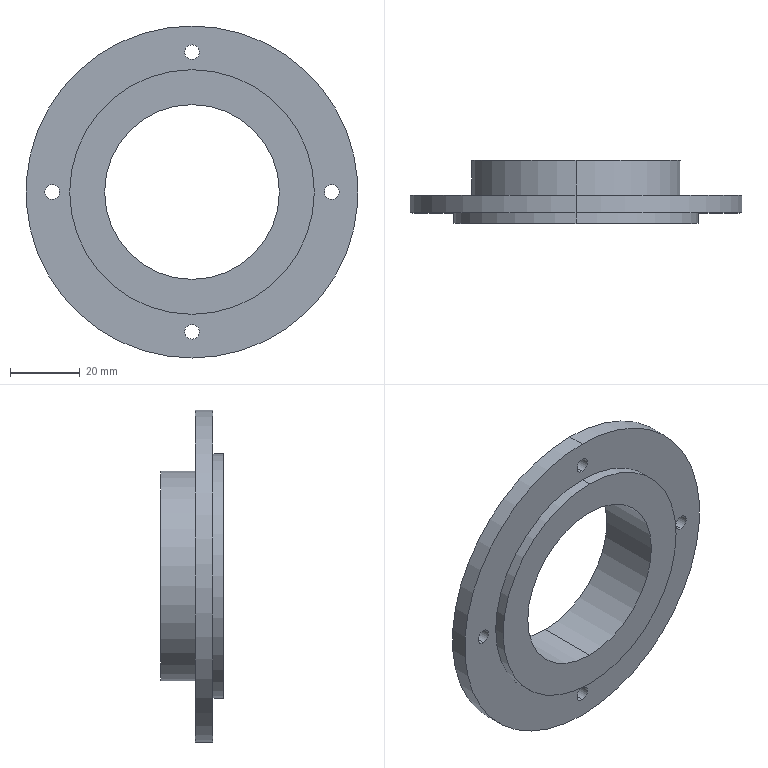Part | STEP file | Rotating Shaft | 1 solid | 20 faces | box 95 x 18 x 95 mm | volume 39641 mm3 | cylinder 16 | plane 4 | commonest cylinder face diameters 4.2 x8 50 x2 60 x2 70 x2 95 x2
STEP:
#1=CARTESIAN_POINT('',(0.,8.,47.5));
#2=VERTEX_POINT('',#1);
#3=CARTESIAN_POINT('',(0.,8.,-47.5));
#4=VERTEX_POINT('',#3);
#5=CARTESIAN_POINT('',(0.,8.,0.));
#6=DIRECTION('',(0.,1.,0.));
#7=DIRECTION('',(0.,0.,-1.));
#8=AXIS2_PLACEMENT_3D('',#5,#6,#7);
#9=CIRCLE('',#8,47.5);
#10=EDGE_CURVE('',#2,#4,#9,.T.);
#11=ORIENTED_EDGE('',*,*,#10,.F.);
#12=CARTESIAN_POINT('',(0.,3.,47.5));
#13=VERTEX_POINT('',#12);
#14=CARTESIAN_POINT('',(0.,0.,47.5));
#15=DIRECTION('',(0.,-1.,0.));
#16=VECTOR('',#15,1000.);
#17=LINE('',#14,#16);
#18=EDGE_CURVE('',#2,#13,#17,.T.);
#19=ORIENTED_EDGE('',*,*,#18,.T.);
#20=CARTESIAN_POINT('',(0.,3.,-47.5));
#21=VERTEX_POINT('',#20);
#22=CARTESIAN_POINT('',(0.,3.,0.));
#23=DIRECTION('',(0.,1.,0.));
#24=DIRECTION('',(0.,0.,-1.));
#25=AXIS2_PLACEMENT_3D('',#22,#23,#24);
#26=CIRCLE('',#25,47.5);
#27=EDGE_CURVE('',#13,#21,#26,.T.);
#28=ORIENTED_EDGE('',*,*,#27,.T.);
#29=CARTESIAN_POINT('',(0.,0.,-47.5));
#30=DIRECTION('',(0.,-1.,0.));
#31=VECTOR('',#30,1000.);
#32=LINE('',#29,#31);
#33=EDGE_CURVE('',#4,#21,#32,.T.);
#34=ORIENTED_EDGE('',*,*,#33,.F.);
#35=EDGE_LOOP('',(#11,#19,#28,#34));
#36=FACE_OUTER_BOUND('',#35,.T.);
#37=CARTESIAN_POINT('',(0.,0.,0.));
#38=DIRECTION('',(0.,-1.,0.));
#39=DIRECTION('',(0.,0.,-1.));
#40=AXIS2_PLACEMENT_3D('',#37,#38,#39);
#41=CYLINDRICAL_SURFACE('',#40,47.5);
#42=ADVANCED_FACE('',(#36),#41,.T.);
#43=CARTESIAN_POINT('',(0.,18.,-30.));
#44=VERTEX_POINT('',#43);
#45=CARTESIAN_POINT('',(0.,18.,30.));
#46=VERTEX_POINT('',#45);
#47=CARTESIAN_POINT('',(0.,18.,0.));
#48=DIRECTION('',(0.,-1.,0.));
#49=DIRECTION('',(0.,0.,-1.));
#50=AXIS2_PLACEMENT_3D('',#47,#48,#49);
#51=CIRCLE('',#50,30.);
#52=EDGE_CURVE('',#44,#46,#51,.T.);
#53=ORIENTED_EDGE('',*,*,#52,.T.);
#54=CARTESIAN_POINT('',(0.,8.,30.));
#55=VERTEX_POINT('',#54);
#56=CARTESIAN_POINT('',(0.,0.,30.));
#57=DIRECTION('',(0.,-1.,0.));
#58=VECTOR('',#57,1000.);
#59=LINE('',#56,#58);
#60=EDGE_CURVE('',#46,#55,#59,.T.);
#61=ORIENTED_EDGE('',*,*,#60,.T.);
#62=CARTESIAN_POINT('',(0.,8.,-30.));
#63=VERTEX_POINT('',#62);
#64=CARTESIAN_POINT('',(0.,8.,0.));
#65=DIRECTION('',(0.,-1.,0.));
#66=DIRECTION('',(0.,0.,-1.));
#67=AXIS2_PLACEMENT_3D('',#64,#65,#66);
#68=CIRCLE('',#67,30.);
#69=EDGE_CURVE('',#63,#55,#68,.T.);
#70=ORIENTED_EDGE('',*,*,#69,.F.);
#71=CARTESIAN_POINT('',(0.,0.,-30.));
#72=DIRECTION('',(0.,-1.,0.));
#73=VECTOR('',#72,1000.);
#74=LINE('',#71,#73);
#75=EDGE_CURVE('',#44,#63,#74,.T.);
#76=ORIENTED_EDGE('',*,*,#75,.F.);
#77=EDGE_LOOP('',(#53,#61,#70,#76));
#78=FACE_OUTER_BOUND('',#77,.T.);
#79=CARTESIAN_POINT('',(0.,0.,0.));
#80=DIRECTION('',(0.,-1.,0.));
#81=DIRECTION('',(0.,0.,-1.));
#82=AXIS2_PLACEMENT_3D('',#79,#80,#81);
#83=CYLINDRICAL_SURFACE('',#82,30.);
#84=ADVANCED_FACE('',(#78),#83,.T.);
#85=CARTESIAN_POINT('',(0.,3.,37.9));
#86=VERTEX_POINT('',#85);
#87=CARTESIAN_POINT('',(0.,3.,42.1));
#88=VERTEX_POINT('',#87);
#89=CARTESIAN_POINT('',(0.,3.,40.));
#90=DIRECTION('',(0.,1.,0.));
#91=DIRECTION('',(0.,0.,1.));
#92=AXIS2_PLACEMENT_3D('',#89,#90,#91);
#93=CIRCLE('',#92,2.1);
#94=EDGE_CURVE('',#86,#88,#93,.T.);
#95=ORIENTED_EDGE('',*,*,#94,.F.);
#96=CARTESIAN_POINT('',(0.,8.,37.9));
#97=VERTEX_POINT('',#96);
#98=CARTESIAN_POINT('',(0.,3.,37.9));
#99=DIRECTION('',(0.,1.,0.));
#100=VECTOR('',#99,1000.);
#101=LINE('',#98,#100);
#102=EDGE_CURVE('',#86,#97,#101,.T.);
#103=ORIENTED_EDGE('',*,*,#102,.T.);
#104=CARTESIAN_POINT('',(0.,8.,42.1));
#105=VERTEX_POINT('',#104);
#106=CARTESIAN_POINT('',(0.,8.,40.));
#107=DIRECTION('',(0.,-1.,0.));
#108=DIRECTION('',(0.,0.,1.));
#109=AXIS2_PLACEMENT_3D('',#106,#107,#108);
#110=CIRCLE('',#109,2.1);
#111=EDGE_CURVE('',#105,#97,#110,.T.);
#112=ORIENTED_EDGE('',*,*,#111,.F.);
#113=CARTESIAN_POINT('',(0.,3.,42.1));
#114=DIRECTION('',(0.,1.,0.));
#115=VECTOR('',#114,1000.);
#116=LINE('',#113,#115);
#117=EDGE_CURVE('',#88,#105,#116,.T.);
#118=ORIENTED_EDGE('',*,*,#117,.F.);
#119=EDGE_LOOP('',(#95,#103,#112,#118));
#120=FACE_OUTER_BOUND('',#119,.T.);
#121=CARTESIAN_POINT('',(0.,3.,40.));
#122=DIRECTION('',(0.,1.,0.));
#123=DIRECTION('',(0.,0.,1.));
#124=AXIS2_PLACEMENT_3D('',#121,#122,#123);
#125=CYLINDRICAL_SURFACE('',#124,2.1);
#126=ADVANCED_FACE('',(#120),#125,.F.);
#127=CARTESIAN_POINT('',(-40.,3.,-2.1));
#128=VERTEX_POINT('',#127);
#129=CARTESIAN_POINT('',(-40.,3.,2.1));
#130=VERTEX_POINT('',#129);
#131=CARTESIAN_POINT('',(-40.,3.,0.));
#132=DIRECTION('',(0.,1.,0.));
#133=DIRECTION('',(0.,0.,1.));
#134=AXIS2_PLACEMENT_3D('',#131,#132,#133);
#135=CIRCLE('',#134,2.1);
#136=EDGE_CURVE('',#128,#130,#135,.T.);
#137=ORIENTED_EDGE('',*,*,#136,.F.);
#138=CARTESIAN_POINT('',(-40.,8.,-2.1));
#139=VERTEX_POINT('',#138);
#140=CARTESIAN_POINT('',(-40.,3.,-2.1));
#141=DIRECTION('',(0.,1.,0.));
#142=VECTOR('',#141,1000.);
#143=LINE('',#140,#142);
#144=EDGE_CURVE('',#128,#139,#143,.T.);
#145=ORIENTED_EDGE('',*,*,#144,.T.);
#146=CARTESIAN_POINT('',(-40.,8.,2.1));
#147=VERTEX_POINT('',#146);
#148=CARTESIAN_POINT('',(-40.,8.,0.));
#149=DIRECTION('',(0.,-1.,0.));
#150=DIRECTION('',(0.,0.,1.));
#151=AXIS2_PLACEMENT_3D('',#148,#149,#150);
#152=CIRCLE('',#151,2.1);
#153=EDGE_CURVE('',#147,#139,#152,.T.);
#154=ORIENTED_EDGE('',*,*,#153,.F.);
#155=CARTESIAN_POINT('',(-40.,3.,2.1));
#156=DIRECTION('',(0.,1.,0.));
#157=VECTOR('',#156,1000.);
#158=LINE('',#155,#157);
#159=EDGE_CURVE('',#130,#147,#158,.T.);
#160=ORIENTED_EDGE('',*,*,#159,.F.);
#161=EDGE_LOOP('',(#137,#145,#154,#160));
#162=FACE_OUTER_BOUND('',#161,.T.);
#163=CARTESIAN_POINT('',(-40.,3.,0.));
#164=DIRECTION('',(0.,1.,0.));
#165=DIRECTION('',(0.,0.,1.));
#166=AXIS2_PLACEMENT_3D('',#163,#164,#165);
#167=CYLINDRICAL_SURFACE('',#166,2.1);
#168=ADVANCED_FACE('',(#162),#167,.F.);
#169=CARTESIAN_POINT('',(0.,3.,-42.1));
#170=VERTEX_POINT('',#169);
#171=CARTESIAN_POINT('',(0.,3.,-37.9));
#172=VERTEX_POINT('',#171);
#173=CARTESIAN_POINT('',(0.,3.,-40.));
#174=DIRECTION('',(0.,1.,0.));
#175=DIRECTION('',(0.,0.,1.));
#176=AXIS2_PLACEMENT_3D('',#173,#174,#175);
#177=CIRCLE('',#176,2.1);
#178=EDGE_CURVE('',#170,#172,#177,.T.);
#179=ORIENTED_EDGE('',*,*,#178,.F.);
#180=CARTESIAN_POINT('',(0.,8.,-42.1));
#181=VERTEX_POINT('',#180);
#182=CARTESIAN_POINT('',(0.,3.,-42.1));
#183=DIRECTION('',(0.,1.,0.));
#184=VECTOR('',#183,1000.);
#185=LINE('',#182,#184);
#186=EDGE_CURVE('',#170,#181,#185,.T.);
#187=ORIENTED_EDGE('',*,*,#186,.T.);
#188=CARTESIAN_POINT('',(0.,8.,-37.9));
#189=VERTEX_POINT('',#188);
#190=CARTESIAN_POINT('',(0.,8.,-40.));
#191=DIRECTION('',(0.,-1.,0.));
#192=DIRECTION('',(0.,0.,1.));
#193=AXIS2_PLACEMENT_3D('',#190,#191,#192);
#194=CIRCLE('',#193,2.1);
#195=EDGE_CURVE('',#189,#181,#194,.T.);
#196=ORIENTED_EDGE('',*,*,#195,.F.);
#197=CARTESIAN_POINT('',(0.,3.,-37.9));
#198=DIRECTION('',(0.,1.,0.));
#199=VECTOR('',#198,1000.);
#200=LINE('',#197,#199);
#201=EDGE_CURVE('',#172,#189,#200,.T.);
#202=ORIENTED_EDGE('',*,*,#201,.F.);
#203=EDGE_LOOP('',(#179,#187,#196,#202));
#204=FACE_OUTER_BOUND('',#203,.T.);
#205=CARTESIAN_POINT('',(0.,3.,-40.));
#206=DIRECTION('',(0.,1.,0.));
#207=DIRECTION('',(0.,0.,1.));
#208=AXIS2_PLACEMENT_3D('',#205,#206,#207);
#209=CYLINDRICAL_SURFACE('',#208,2.1);
#210=ADVANCED_FACE('',(#204),#209,.F.);
#211=CARTESIAN_POINT('',(40.,3.,-2.1));
#212=VERTEX_POINT('',#211);
#213=CARTESIAN_POINT('',(40.,3.,2.1));
#214=VERTEX_POINT('',#213);
#215=CARTESIAN_POINT('',(40.,3.,0.));
#216=DIRECTION('',(0.,1.,0.));
#217=DIRECTION('',(0.,0.,1.));
#218=AXIS2_PLACEMENT_3D('',#215,#216,#217);
#219=CIRCLE('',#218,2.1);
#220=EDGE_CURVE('',#212,#214,#219,.T.);
#221=ORIENTED_EDGE('',*,*,#220,.F.);
#222=CARTESIAN_POINT('',(40.,8.,-2.1));
#223=VERTEX_POINT('',#222);
#224=CARTESIAN_POINT('',(40.,3.,-2.1));
#225=DIRECTION('',(0.,1.,0.));
#226=VECTOR('',#225,1000.);
#227=LINE('',#224,#226);
#228=EDGE_CURVE('',#212,#223,#227,.T.);
#229=ORIENTED_EDGE('',*,*,#228,.T.);
#230=CARTESIAN_POINT('',(40.,8.,2.1));
#231=VERTEX_POINT('',#230);
#232=CARTESIAN_POINT('',(40.,8.,0.));
#233=DIRECTION('',(0.,-1.,0.));
#234=DIRECTION('',(0.,0.,1.));
#235=AXIS2_PLACEMENT_3D('',#232,#233,#234);
#236=CIRCLE('',#235,2.1);
#237=EDGE_CURVE('',#231,#223,#236,.T.);
#238=ORIENTED_EDGE('',*,*,#237,.F.);
#239=CARTESIAN_POINT('',(40.,3.,2.1));
#240=DIRECTION('',(0.,1.,0.));
#241=VECTOR('',#240,1000.);
#242=LINE('',#239,#241);
#243=EDGE_CURVE('',#214,#231,#242,.T.);
#244=ORIENTED_EDGE('',*,*,#243,.F.);
#245=EDGE_LOOP('',(#221,#229,#238,#244));
#246=FACE_OUTER_BOUND('',#245,.T.);
#247=CARTESIAN_POINT('',(40.,3.,0.));
#248=DIRECTION('',(0.,1.,0.));
#249=DIRECTION('',(0.,0.,1.));
#250=AXIS2_PLACEMENT_3D('',#247,#248,#249);
#251=CYLINDRICAL_SURFACE('',#250,2.1);
#252=ADVANCED_FACE('',(#246),#251,.F.);
#253=CARTESIAN_POINT('',(0.,3.,35.));
#254=VERTEX_POINT('',#253);
#255=CARTESIAN_POINT('',(0.,3.,-35.));
#256=VERTEX_POINT('',#255);
#257=CARTESIAN_POINT('',(0.,3.,0.));
#258=DIRECTION('',(0.,1.,0.));
#259=DIRECTION('',(0.,0.,-1.));
#260=AXIS2_PLACEMENT_3D('',#257,#258,#259);
#261=CIRCLE('',#260,35.);
#262=EDGE_CURVE('',#254,#256,#261,.T.);
#263=ORIENTED_EDGE('',*,*,#262,.F.);
#264=CARTESIAN_POINT('',(0.,0.,35.));
#265=VERTEX_POINT('',#264);
#266=CARTESIAN_POINT('',(0.,0.,35.));
#267=DIRECTION('',(0.,-1.,0.));
#268=VECTOR('',#267,1000.);
#269=LINE('',#266,#268);
#270=EDGE_CURVE('',#254,#265,#269,.T.);
#271=ORIENTED_EDGE('',*,*,#270,.T.);
#272=CARTESIAN_POINT('',(0.,0.,-35.));
#273=VERTEX_POINT('',#272);
#274=CARTESIAN_POINT('',(0.,0.,0.));
#275=DIRECTION('',(0.,1.,0.));
#276=DIRECTION('',(0.,0.,-1.));
#277=AXIS2_PLACEMENT_3D('',#274,#275,#276);
#278=CIRCLE('',#277,35.);
#279=EDGE_CURVE('',#265,#273,#278,.T.);
#280=ORIENTED_EDGE('',*,*,#279,.T.);
#281=CARTESIAN_POINT('',(0.,0.,-35.));
#282=DIRECTION('',(0.,-1.,0.));
#283=VECTOR('',#282,1000.);
#284=LINE('',#281,#283);
#285=EDGE_CURVE('',#256,#273,#284,.T.);
#286=ORIENTED_EDGE('',*,*,#285,.F.);
#287=EDGE_LOOP('',(#263,#271,#280,#286));
#288=FACE_OUTER_BOUND('',#287,.T.);
#289=CARTESIAN_POINT('',(0.,0.,0.));
#290=DIRECTION('',(0.,-1.,0.));
#291=DIRECTION('',(0.,0.,-1.));
#292=AXIS2_PLACEMENT_3D('',#289,#290,#291);
#293=CYLINDRICAL_SURFACE('',#292,35.);
#294=ADVANCED_FACE('',(#288),#293,.T.);
#295=CARTESIAN_POINT('',(0.,18.,25.));
#296=VERTEX_POINT('',#295);
#297=CARTESIAN_POINT('',(0.,18.,-25.));
#298=VERTEX_POINT('',#297);
#299=CARTESIAN_POINT('',(0.,18.,0.));
#300=DIRECTION('',(0.,-1.,0.));
#301=DIRECTION('',(0.,0.,-1.));
#302=AXIS2_PLACEMENT_3D('',#299,#300,#301);
#303=CIRCLE('',#302,25.);
#304=EDGE_CURVE('',#296,#298,#303,.T.);
#305=ORIENTED_EDGE('',*,*,#304,.F.);
#306=CARTESIAN_POINT('',(0.,0.,25.));
#307=VERTEX_POINT('',#306);
#308=CARTESIAN_POINT('',(0.,0.,25.));
#309=DIRECTION('',(0.,-1.,0.));
#310=VECTOR('',#309,1000.);
#311=LINE('',#308,#310);
#312=EDGE_CURVE('',#296,#307,#311,.T.);
#313=ORIENTED_EDGE('',*,*,#312,.T.);
#314=CARTESIAN_POINT('',(0.,0.,-25.));
#315=VERTEX_POINT('',#314);
#316=CARTESIAN_POINT('',(0.,0.,0.));
#317=DIRECTION('',(0.,1.,0.));
#318=DIRECTION('',(0.,0.,-1.));
#319=AXIS2_PLACEMENT_3D('',#316,#317,#318);
#320=CIRCLE('',#319,25.);
#321=EDGE_CURVE('',#315,#307,#320,.T.);
#322=ORIENTED_EDGE('',*,*,#321,.F.);
#323=CARTESIAN_POINT('',(0.,0.,-25.));
#324=DIRECTION('',(0.,-1.,0.));
#325=VECTOR('',#324,1000.);
#326=LINE('',#323,#325);
#327=EDGE_CURVE('',#298,#315,#326,.T.);
#328=ORIENTED_EDGE('',*,*,#327,.F.);
#329=EDGE_LOOP('',(#305,#313,#322,#328));
#330=FACE_OUTER_BOUND('',#329,.T.);
#331=CARTESIAN_POINT('',(0.,0.,0.));
#332=DIRECTION('',(0.,-1.,0.));
#333=DIRECTION('',(0.,0.,-1.));
#334=AXIS2_PLACEMENT_3D('',#331,#332,#333);
#335=CYLINDRICAL_SURFACE('',#334,25.);
#336=ADVANCED_FACE('',(#330),#335,.F.);
#337=CARTESIAN_POINT('',(0.,8.,0.));
#338=DIRECTION('',(0.,1.,0.));
#339=DIRECTION('',(0.,0.,-1.));
#340=AXIS2_PLACEMENT_3D('',#337,#338,#339);
#341=CIRCLE('',#340,47.5);
#342=EDGE_CURVE('',#4,#2,#341,.T.);
#343=ORIENTED_EDGE('',*,*,#342,.T.);
#344=ORIENTED_EDGE('',*,*,#10,.T.);
#345=EDGE_LOOP('',(#343,#344));
#346=FACE_OUTER_BOUND('',#345,.T.);
#347=ORIENTED_EDGE('',*,*,#69,.T.);
#348=CARTESIAN_POINT('',(0.,8.,0.));
#349=DIRECTION('',(0.,-1.,0.));
#350=DIRECTION('',(0.,0.,-1.));
#351=AXIS2_PLACEMENT_3D('',#348,#349,#350);
#352=CIRCLE('',#351,30.);
#353=EDGE_CURVE('',#55,#63,#352,.T.);
#354=ORIENTED_EDGE('',*,*,#353,.T.);
#355=EDGE_LOOP('',(#347,#354));
#356=FACE_BOUND('',#355,.T.);
#357=ORIENTED_EDGE('',*,*,#111,.T.);
#358=CARTESIAN_POINT('',(0.,8.,40.));
#359=DIRECTION('',(0.,-1.,0.));
#360=DIRECTION('',(0.,0.,1.));
#361=AXIS2_PLACEMENT_3D('',#358,#359,#360);
#362=CIRCLE('',#361,2.1);
#363=EDGE_CURVE('',#97,#105,#362,.T.);
#364=ORIENTED_EDGE('',*,*,#363,.T.);
#365=EDGE_LOOP('',(#357,#364));
#366=FACE_BOUND('',#365,.T.);
#367=ORIENTED_EDGE('',*,*,#153,.T.);
#368=CARTESIAN_POINT('',(-40.,8.,0.));
#369=DIRECTION('',(0.,-1.,0.));
#370=DIRECTION('',(0.,0.,1.));
#371=AXIS2_PLACEMENT_3D('',#368,#369,#370);
#372=CIRCLE('',#371,2.1);
#373=EDGE_CURVE('',#139,#147,#372,.T.);
#374=ORIENTED_EDGE('',*,*,#373,.T.);
#375=EDGE_LOOP('',(#367,#374));
#376=FACE_BOUND('',#375,.T.);
#377=ORIENTED_EDGE('',*,*,#195,.T.);
#378=CARTESIAN_POINT('',(0.,8.,-40.));
#379=DIRECTION('',(0.,-1.,0.));
#380=DIRECTION('',(0.,0.,1.));
#381=AXIS2_PLACEMENT_3D('',#378,#379,#380);
#382=CIRCLE('',#381,2.1);
#383=EDGE_CURVE('',#181,#189,#382,.T.);
#384=ORIENTED_EDGE('',*,*,#383,.T.);
#385=EDGE_LOOP('',(#377,#384));
#386=FACE_BOUND('',#385,.T.);
#387=ORIENTED_EDGE('',*,*,#237,.T.);
#388=CARTESIAN_POINT('',(40.,8.,0.));
#389=DIRECTION('',(0.,-1.,0.));
#390=DIRECTION('',(0.,0.,1.));
#391=AXIS2_PLACEMENT_3D('',#388,#389,#390);
#392=CIRCLE('',#391,2.1);
#393=EDGE_CURVE('',#223,#231,#392,.T.);
#394=ORIENTED_EDGE('',*,*,#393,.T.);
#395=EDGE_LOOP('',(#387,#394));
#396=FACE_BOUND('',#395,.T.);
#397=CARTESIAN_POINT('',(47.5,8.,0.));
#398=DIRECTION('',(0.,1.,0.));
#399=DIRECTION('',(0.,0.,1.));
#400=AXIS2_PLACEMENT_3D('',#397,#398,#399);
#401=PLANE('',#400);
#402=ADVANCED_FACE('',(#346,#356,#366,#376,#386,#396),#401,.T.);
#403=ORIENTED_EDGE('',*,*,#18,.F.);
#404=ORIENTED_EDGE('',*,*,#342,.F.);
#405=ORIENTED_EDGE('',*,*,#33,.T.);
#406=CARTESIAN_POINT('',(0.,3.,0.));
#407=DIRECTION('',(0.,1.,0.));
#408=DIRECTION('',(0.,0.,-1.));
#409=AXIS2_PLACEMENT_3D('',#406,#407,#408);
#410=CIRCLE('',#409,47.5);
#411=EDGE_CURVE('',#21,#13,#410,.T.);
#412=ORIENTED_EDGE('',*,*,#411,.T.);
#413=EDGE_LOOP('',(#403,#404,#405,#412));
#414=FACE_OUTER_BOUND('',#413,.T.);
#415=CARTESIAN_POINT('',(0.,0.,0.));
#416=DIRECTION('',(0.,-1.,0.));
#417=DIRECTION('',(0.,0.,-1.));
#418=AXIS2_PLACEMENT_3D('',#415,#416,#417);
#419=CYLINDRICAL_SURFACE('',#418,47.5);
#420=ADVANCED_FACE('',(#414),#419,.T.);
#421=ORIENTED_EDGE('',*,*,#60,.F.);
#422=CARTESIAN_POINT('',(0.,18.,0.));
#423=DIRECTION('',(0.,-1.,0.));
#424=DIRECTION('',(0.,0.,-1.));
#425=AXIS2_PLACEMENT_3D('',#422,#423,#424);
#426=CIRCLE('',#425,30.);
#427=EDGE_CURVE('',#46,#44,#426,.T.);
#428=ORIENTED_EDGE('',*,*,#427,.T.);
#429=ORIENTED_EDGE('',*,*,#75,.T.);
#430=ORIENTED_EDGE('',*,*,#353,.F.);
#431=EDGE_LOOP('',(#421,#428,#429,#430));
#432=FACE_OUTER_BOUND('',#431,.T.);
#433=CARTESIAN_POINT('',(0.,0.,0.));
#434=DIRECTION('',(0.,-1.,0.));
#435=DIRECTION('',(0.,0.,-1.));
#436=AXIS2_PLACEMENT_3D('',#433,#434,#435);
#437=CYLINDRICAL_SURFACE('',#436,30.);
#438=ADVANCED_FACE('',(#432),#437,.T.);
#439=ORIENTED_EDGE('',*,*,#102,.F.);
#440=CARTESIAN_POINT('',(0.,3.,40.));
#441=DIRECTION('',(0.,1.,0.));
#442=DIRECTION('',(0.,0.,1.));
#443=AXIS2_PLACEMENT_3D('',#440,#441,#442);
#444=CIRCLE('',#443,2.1);
#445=EDGE_CURVE('',#88,#86,#444,.T.);
#446=ORIENTED_EDGE('',*,*,#445,.F.);
#447=ORIENTED_EDGE('',*,*,#117,.T.);
#448=ORIENTED_EDGE('',*,*,#363,.F.);
#449=EDGE_LOOP('',(#439,#446,#447,#448));
#450=FACE_OUTER_BOUND('',#449,.T.);
#451=CARTESIAN_POINT('',(0.,3.,40.));
#452=DIRECTION('',(0.,1.,0.));
#453=DIRECTION('',(0.,0.,1.));
#454=AXIS2_PLACEMENT_3D('',#451,#452,#453);
#455=CYLINDRICAL_SURFACE('',#454,2.1);
#456=ADVANCED_FACE('',(#450),#455,.F.);
#457=ORIENTED_EDGE('',*,*,#144,.F.);
#458=CARTESIAN_POINT('',(-40.,3.,0.));
#459=DIRECTION('',(0.,1.,0.));
#460=DIRECTION('',(0.,0.,1.));
#461=AXIS2_PLACEMENT_3D('',#458,#459,#460);
#462=CIRCLE('',#461,2.1);
#463=EDGE_CURVE('',#130,#128,#462,.T.);
#464=ORIENTED_EDGE('',*,*,#463,.F.);
#465=ORIENTED_EDGE('',*,*,#159,.T.);
#466=ORIENTED_EDGE('',*,*,#373,.F.);
#467=EDGE_LOOP('',(#457,#464,#465,#466));
#468=FACE_OUTER_BOUND('',#467,.T.);
#469=CARTESIAN_POINT('',(-40.,3.,0.));
#470=DIRECTION('',(0.,1.,0.));
#471=DIRECTION('',(0.,0.,1.));
#472=AXIS2_PLACEMENT_3D('',#469,#470,#471);
#473=CYLINDRICAL_SURFACE('',#472,2.1);
#474=ADVANCED_FACE('',(#468),#473,.F.);
#475=ORIENTED_EDGE('',*,*,#186,.F.);
#476=CARTESIAN_POINT('',(0.,3.,-40.));
#477=DIRECTION('',(0.,1.,0.));
#478=DIRECTION('',(0.,0.,1.));
#479=AXIS2_PLACEMENT_3D('',#476,#477,#478);
#480=CIRCLE('',#479,2.1);
#481=EDGE_CURVE('',#172,#170,#480,.T.);
#482=ORIENTED_EDGE('',*,*,#481,.F.);
#483=ORIENTED_EDGE('',*,*,#201,.T.);
#484=ORIENTED_EDGE('',*,*,#383,.F.);
#485=EDGE_LOOP('',(#475,#482,#483,#484));
#486=FACE_OUTER_BOUND('',#485,.T.);
#487=CARTESIAN_POINT('',(0.,3.,-40.));
#488=DIRECTION('',(0.,1.,0.));
#489=DIRECTION('',(0.,0.,1.));
#490=AXIS2_PLACEMENT_3D('',#487,#488,#489);
#491=CYLINDRICAL_SURFACE('',#490,2.1);
#492=ADVANCED_FACE('',(#486),#491,.F.);
#493=ORIENTED_EDGE('',*,*,#228,.F.);
#494=CARTESIAN_POINT('',(40.,3.,0.));
#495=DIRECTION('',(0.,1.,0.));
#496=DIRECTION('',(0.,0.,1.));
#497=AXIS2_PLACEMENT_3D('',#494,#495,#496);
#498=CIRCLE('',#497,2.1);
#499=EDGE_CURVE('',#214,#212,#498,.T.);
#500=ORIENTED_EDGE('',*,*,#499,.F.);
#501=ORIENTED_EDGE('',*,*,#243,.T.);
#502=ORIENTED_EDGE('',*,*,#393,.F.);
#503=EDGE_LOOP('',(#493,#500,#501,#502));
#504=FACE_OUTER_BOUND('',#503,.T.);
#505=CARTESIAN_POINT('',(40.,3.,0.));
#506=DIRECTION('',(0.,1.,0.));
#507=DIRECTION('',(0.,0.,1.));
#508=AXIS2_PLACEMENT_3D('',#505,#506,#507);
#509=CYLINDRICAL_SURFACE('',#508,2.1);
#510=ADVANCED_FACE('',(#504),#509,.F.);
#511=CARTESIAN_POINT('',(0.,3.,0.));
#512=DIRECTION('',(0.,1.,0.));
#513=DIRECTION('',(0.,0.,-1.));
#514=AXIS2_PLACEMENT_3D('',#511,#512,#513);
#515=CIRCLE('',#514,35.);
#516=EDGE_CURVE('',#256,#254,#515,.T.);
#517=ORIENTED_EDGE('',*,*,#516,.T.);
#518=ORIENTED_EDGE('',*,*,#262,.T.);
#519=EDGE_LOOP('',(#517,#518));
#520=FACE_BOUND('',#519,.T.);
#521=ORIENTED_EDGE('',*,*,#411,.F.);
#522=ORIENTED_EDGE('',*,*,#27,.F.);
#523=EDGE_LOOP('',(#521,#522));
#524=FACE_OUTER_BOUND('',#523,.T.);
#525=ORIENTED_EDGE('',*,*,#445,.T.);
#526=ORIENTED_EDGE('',*,*,#94,.T.);
#527=EDGE_LOOP('',(#525,#526));
#528=FACE_BOUND('',#527,.T.);
#529=ORIENTED_EDGE('',*,*,#463,.T.);
#530=ORIENTED_EDGE('',*,*,#136,.T.);
#531=EDGE_LOOP('',(#529,#530));
#532=FACE_BOUND('',#531,.T.);
#533=ORIENTED_EDGE('',*,*,#481,.T.);
#534=ORIENTED_EDGE('',*,*,#178,.T.);
#535=EDGE_LOOP('',(#533,#534));
#536=FACE_BOUND('',#535,.T.);
#537=ORIENTED_EDGE('',*,*,#499,.T.);
#538=ORIENTED_EDGE('',*,*,#220,.T.);
#539=EDGE_LOOP('',(#537,#538));
#540=FACE_BOUND('',#539,.T.);
#541=CARTESIAN_POINT('',(35.,3.,0.));
#542=DIRECTION('',(0.,-1.,0.));
#543=DIRECTION('',(0.,0.,-1.));
#544=AXIS2_PLACEMENT_3D('',#541,#542,#543);
#545=PLANE('',#544);
#546=ADVANCED_FACE('',(#520,#524,#528,#532,#536,#540),#545,.T.);
#547=ORIENTED_EDGE('',*,*,#52,.F.);
#548=ORIENTED_EDGE('',*,*,#427,.F.);
#549=EDGE_LOOP('',(#547,#548));
#550=FACE_OUTER_BOUND('',#549,.T.);
#551=CARTESIAN_POINT('',(0.,18.,0.));
#552=DIRECTION('',(0.,-1.,0.));
#553=DIRECTION('',(0.,0.,-1.));
#554=AXIS2_PLACEMENT_3D('',#551,#552,#553);
#555=CIRCLE('',#554,25.);
#556=EDGE_CURVE('',#298,#296,#555,.T.);
#557=ORIENTED_EDGE('',*,*,#556,.T.);
#558=ORIENTED_EDGE('',*,*,#304,.T.);
#559=EDGE_LOOP('',(#557,#558));
#560=FACE_BOUND('',#559,.T.);
#561=CARTESIAN_POINT('',(30.,18.,0.));
#562=DIRECTION('',(0.,1.,0.));
#563=DIRECTION('',(0.,0.,1.));
#564=AXIS2_PLACEMENT_3D('',#561,#562,#563);
#565=PLANE('',#564);
#566=ADVANCED_FACE('',(#550,#560),#565,.T.);
#567=ORIENTED_EDGE('',*,*,#270,.F.);
#568=ORIENTED_EDGE('',*,*,#516,.F.);
#569=ORIENTED_EDGE('',*,*,#285,.T.);
#570=CARTESIAN_POINT('',(0.,0.,0.));
#571=DIRECTION('',(0.,1.,0.));
#572=DIRECTION('',(0.,0.,-1.));
#573=AXIS2_PLACEMENT_3D('',#570,#571,#572);
#574=CIRCLE('',#573,35.);
#575=EDGE_CURVE('',#273,#265,#574,.T.);
#576=ORIENTED_EDGE('',*,*,#575,.T.);
#577=EDGE_LOOP('',(#567,#568,#569,#576));
#578=FACE_OUTER_BOUND('',#577,.T.);
#579=CARTESIAN_POINT('',(0.,0.,0.));
#580=DIRECTION('',(0.,-1.,0.));
#581=DIRECTION('',(0.,0.,-1.));
#582=AXIS2_PLACEMENT_3D('',#579,#580,#581);
#583=CYLINDRICAL_SURFACE('',#582,35.);
#584=ADVANCED_FACE('',(#578),#583,.T.);
#585=ORIENTED_EDGE('',*,*,#312,.F.);
#586=ORIENTED_EDGE('',*,*,#556,.F.);
#587=ORIENTED_EDGE('',*,*,#327,.T.);
#588=CARTESIAN_POINT('',(0.,0.,0.));
#589=DIRECTION('',(0.,1.,0.));
#590=DIRECTION('',(0.,0.,-1.));
#591=AXIS2_PLACEMENT_3D('',#588,#589,#590);
#592=CIRCLE('',#591,25.);
#593=EDGE_CURVE('',#307,#315,#592,.T.);
#594=ORIENTED_EDGE('',*,*,#593,.F.);
#595=EDGE_LOOP('',(#585,#586,#587,#594));
#596=FACE_OUTER_BOUND('',#595,.T.);
#597=CARTESIAN_POINT('',(0.,0.,0.));
#598=DIRECTION('',(0.,-1.,0.));
#599=DIRECTION('',(0.,0.,-1.));
#600=AXIS2_PLACEMENT_3D('',#597,#598,#599);
#601=CYLINDRICAL_SURFACE('',#600,25.);
#602=ADVANCED_FACE('',(#596),#601,.F.);
#603=ORIENTED_EDGE('',*,*,#321,.T.);
#604=ORIENTED_EDGE('',*,*,#593,.T.);
#605=EDGE_LOOP('',(#603,#604));
#606=FACE_BOUND('',#605,.T.);
#607=ORIENTED_EDGE('',*,*,#575,.F.);
#608=ORIENTED_EDGE('',*,*,#279,.F.);
#609=EDGE_LOOP('',(#607,#608));
#610=FACE_OUTER_BOUND('',#609,.T.);
#611=CARTESIAN_POINT('',(25.,0.,0.));
#612=DIRECTION('',(0.,-1.,0.));
#613=DIRECTION('',(0.,0.,-1.));
#614=AXIS2_PLACEMENT_3D('',#611,#612,#613);
#615=PLANE('',#614);
#616=ADVANCED_FACE('',(#606,#610),#615,.T.);
#617=CLOSED_SHELL('',(#42,#84,#126,#168,#210,#252,#294,#336,#402,#420,#438,#456,#474,#492,#510,#546,#566,#584,#602,#616));
#618=MANIFOLD_SOLID_BREP('',#617);
#619=CARTESIAN_POINT('',(0.,0.,0.));
#620=DIRECTION('',(0.,0.,1.));
#621=DIRECTION('',(1.,0.,0.));
#622=AXIS2_PLACEMENT_3D('',#619,#620,#621);
#623=(LENGTH_UNIT()NAMED_UNIT(*)SI_UNIT(.MILLI.,.METRE.));
#624=UNCERTAINTY_MEASURE_WITH_UNIT(LENGTH_MEASURE(0.00001),#623,'','');
#625=(NAMED_UNIT(*)PLANE_ANGLE_UNIT()SI_UNIT($,.RADIAN.));
#626=(NAMED_UNIT(*)SI_UNIT($,.STERADIAN.)SOLID_ANGLE_UNIT());
#627=(GEOMETRIC_REPRESENTATION_CONTEXT(3)GLOBAL_UNCERTAINTY_ASSIGNED_CONTEXT((#624))GLOBAL_UNIT_ASSIGNED_CONTEXT((#623,#625,#626))REPRESENTATION_CONTEXT('',''));
#628=ADVANCED_BREP_SHAPE_REPRESENTATION('',(#618,#622),#627);